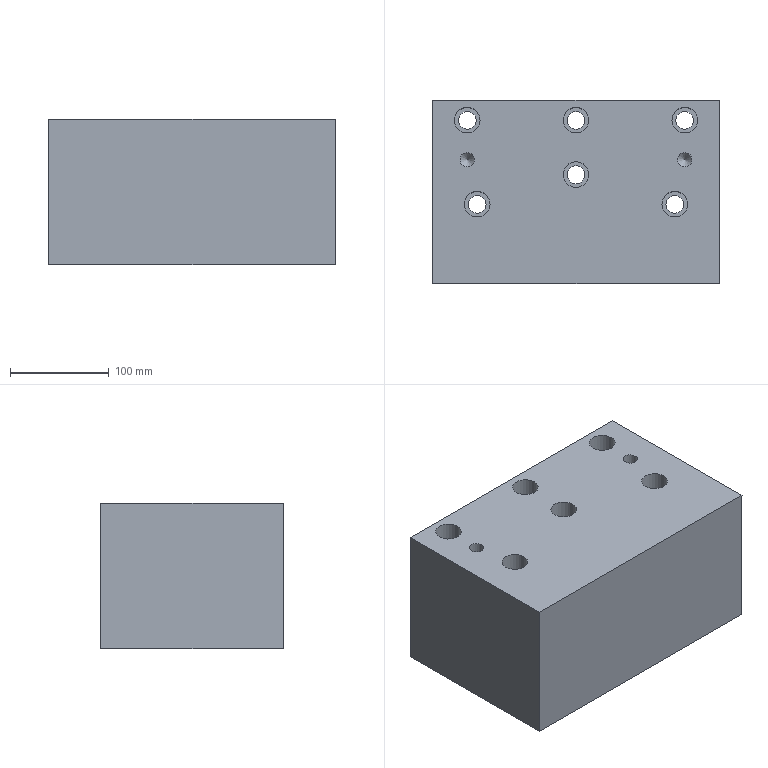Part | STEP file | lll_id2190_x_t | 1 solid | 32 faces | box 290 x 185 x 147.5 mm | volume 7467987 mm3 | cylinder 16 | plane 12 | cone 4 | commonest cylinder face diameters 18.009 x6 26.008 x6 14.506 x4
STEP:
#1=CARTESIAN_POINT('',(1973.431,-495.,262.5));
#2=VERTEX_POINT('',#1);
#3=CARTESIAN_POINT('',(1982.435,-495.,262.5));
#4=DIRECTION('',(0.,0.,-1.));
#5=DIRECTION('',(-1.,0.,0.));
#6=AXIS2_PLACEMENT_3D('',#3,#4,#5);
#7=CIRCLE('',#6,9.005);
#8=EDGE_CURVE('',#2,#2,#7,.T.);
#9=ORIENTED_EDGE('',*,*,#8,.T.);
#10=EDGE_LOOP('',(#9));
#11=FACE_BOUND('',#10,.T.);
#12=CARTESIAN_POINT('',(1995.439,-495.,262.5));
#13=VERTEX_POINT('',#12);
#14=CARTESIAN_POINT('',(1982.435,-495.,262.5));
#15=DIRECTION('',(0.,0.,-1.));
#16=DIRECTION('',(1.,0.,0.));
#17=AXIS2_PLACEMENT_3D('',#14,#15,#16);
#18=CIRCLE('',#17,13.004);
#19=EDGE_CURVE('',#13,#13,#18,.T.);
#20=ORIENTED_EDGE('',*,*,#19,.F.);
#21=EDGE_LOOP('',(#20));
#22=FACE_BOUND('',#21,.T.);
#23=CARTESIAN_POINT('',(1982.435,-495.,262.5));
#24=DIRECTION('',(0.,0.,-1.));
#25=DIRECTION('',(-1.,0.,0.));
#26=AXIS2_PLACEMENT_3D('',#23,#24,#25);
#27=PLANE('',#26);
#28=ADVANCED_FACE('',(#11,#22),#27,.F.);
#29=CARTESIAN_POINT('',(1983.431,-580.,262.5));
#30=VERTEX_POINT('',#29);
#31=CARTESIAN_POINT('',(1992.435,-580.,262.5));
#32=DIRECTION('',(0.,0.,-1.));
#33=DIRECTION('',(-1.,0.,0.));
#34=AXIS2_PLACEMENT_3D('',#31,#32,#33);
#35=CIRCLE('',#34,9.005);
#36=EDGE_CURVE('',#30,#30,#35,.T.);
#37=ORIENTED_EDGE('',*,*,#36,.T.);
#38=EDGE_LOOP('',(#37));
#39=FACE_BOUND('',#38,.T.);
#40=CARTESIAN_POINT('',(2005.439,-580.,262.5));
#41=VERTEX_POINT('',#40);
#42=CARTESIAN_POINT('',(1992.435,-580.,262.5));
#43=DIRECTION('',(0.,0.,-1.));
#44=DIRECTION('',(1.,0.,0.));
#45=AXIS2_PLACEMENT_3D('',#42,#43,#44);
#46=CIRCLE('',#45,13.004);
#47=EDGE_CURVE('',#41,#41,#46,.T.);
#48=ORIENTED_EDGE('',*,*,#47,.F.);
#49=EDGE_LOOP('',(#48));
#50=FACE_BOUND('',#49,.T.);
#51=CARTESIAN_POINT('',(1992.435,-580.,262.5));
#52=DIRECTION('',(0.,0.,-1.));
#53=DIRECTION('',(-1.,0.,0.));
#54=AXIS2_PLACEMENT_3D('',#51,#52,#53);
#55=PLANE('',#54);
#56=ADVANCED_FACE('',(#39,#50),#55,.F.);
#57=CARTESIAN_POINT('',(1982.435,-535.,279.494));
#58=VERTEX_POINT('',#57);
#59=VERTEX_LOOP('',#58);
#60=FACE_BOUND('',#59,.T.);
#61=CARTESIAN_POINT('',(1989.688,-535.,286.747));
#62=VERTEX_POINT('',#61);
#63=CARTESIAN_POINT('',(1982.435,-535.,286.747));
#64=DIRECTION('',(0.,0.,-1.));
#65=DIRECTION('',(1.,0.,0.));
#66=AXIS2_PLACEMENT_3D('',#63,#64,#65);
#67=CIRCLE('',#66,7.253);
#68=EDGE_CURVE('',#62,#62,#67,.T.);
#69=ORIENTED_EDGE('',*,*,#68,.F.);
#70=EDGE_LOOP('',(#69));
#71=FACE_BOUND('',#70,.T.);
#72=CARTESIAN_POINT('',(1982.435,-535.,286.747));
#73=DIRECTION('',(0.,0.,1.));
#74=DIRECTION('',(-1.,0.,0.));
#75=AXIS2_PLACEMENT_3D('',#72,#73,#74);
#76=CONICAL_SURFACE('',#75,7.253,45.);
#77=ADVANCED_FACE('',(#60,#71),#76,.F.);
#78=CARTESIAN_POINT('',(2202.435,-535.,279.494));
#79=VERTEX_POINT('',#78);
#80=VERTEX_LOOP('',#79);
#81=FACE_BOUND('',#80,.T.);
#82=CARTESIAN_POINT('',(2195.182,-535.,286.747));
#83=VERTEX_POINT('',#82);
#84=CARTESIAN_POINT('',(2202.435,-535.,286.747));
#85=DIRECTION('',(0.,0.,-1.));
#86=DIRECTION('',(-1.,0.,0.));
#87=AXIS2_PLACEMENT_3D('',#84,#85,#86);
#88=CIRCLE('',#87,7.253);
#89=EDGE_CURVE('',#83,#83,#88,.T.);
#90=ORIENTED_EDGE('',*,*,#89,.F.);
#91=EDGE_LOOP('',(#90));
#92=FACE_BOUND('',#91,.T.);
#93=CARTESIAN_POINT('',(2202.435,-535.,286.747));
#94=DIRECTION('',(0.,0.,1.));
#95=DIRECTION('',(1.,0.,0.));
#96=AXIS2_PLACEMENT_3D('',#93,#94,#95);
#97=CONICAL_SURFACE('',#96,7.253,45.);
#98=ADVANCED_FACE('',(#81,#92),#97,.F.);
#99=CARTESIAN_POINT('',(2211.44,-495.,262.5));
#100=VERTEX_POINT('',#99);
#101=CARTESIAN_POINT('',(2202.435,-495.,262.5));
#102=DIRECTION('',(0.,0.,-1.));
#103=DIRECTION('',(1.,0.,0.));
#104=AXIS2_PLACEMENT_3D('',#101,#102,#103);
#105=CIRCLE('',#104,9.005);
#106=EDGE_CURVE('',#100,#100,#105,.T.);
#107=ORIENTED_EDGE('',*,*,#106,.T.);
#108=EDGE_LOOP('',(#107));
#109=FACE_BOUND('',#108,.T.);
#110=CARTESIAN_POINT('',(2189.431,-495.,262.5));
#111=VERTEX_POINT('',#110);
#112=CARTESIAN_POINT('',(2202.435,-495.,262.5));
#113=DIRECTION('',(0.,0.,-1.));
#114=DIRECTION('',(-1.,0.,0.));
#115=AXIS2_PLACEMENT_3D('',#112,#113,#114);
#116=CIRCLE('',#115,13.004);
#117=EDGE_CURVE('',#111,#111,#116,.T.);
#118=ORIENTED_EDGE('',*,*,#117,.F.);
#119=EDGE_LOOP('',(#118));
#120=FACE_BOUND('',#119,.T.);
#121=CARTESIAN_POINT('',(2202.435,-495.,262.5));
#122=DIRECTION('',(0.,0.,-1.));
#123=DIRECTION('',(1.,0.,0.));
#124=AXIS2_PLACEMENT_3D('',#121,#122,#123);
#125=PLANE('',#124);
#126=ADVANCED_FACE('',(#109,#120),#125,.F.);
#127=CARTESIAN_POINT('',(2201.44,-580.,262.5));
#128=VERTEX_POINT('',#127);
#129=CARTESIAN_POINT('',(2192.435,-580.,262.5));
#130=DIRECTION('',(0.,0.,-1.));
#131=DIRECTION('',(1.,0.,0.));
#132=AXIS2_PLACEMENT_3D('',#129,#130,#131);
#133=CIRCLE('',#132,9.005);
#134=EDGE_CURVE('',#128,#128,#133,.T.);
#135=ORIENTED_EDGE('',*,*,#134,.T.);
#136=EDGE_LOOP('',(#135));
#137=FACE_BOUND('',#136,.T.);
#138=CARTESIAN_POINT('',(2179.431,-580.,262.5));
#139=VERTEX_POINT('',#138);
#140=CARTESIAN_POINT('',(2192.435,-580.,262.5));
#141=DIRECTION('',(0.,0.,-1.));
#142=DIRECTION('',(-1.,0.,0.));
#143=AXIS2_PLACEMENT_3D('',#140,#141,#142);
#144=CIRCLE('',#143,13.004);
#145=EDGE_CURVE('',#139,#139,#144,.T.);
#146=ORIENTED_EDGE('',*,*,#145,.F.);
#147=EDGE_LOOP('',(#146));
#148=FACE_BOUND('',#147,.T.);
#149=CARTESIAN_POINT('',(2192.435,-580.,262.5));
#150=DIRECTION('',(0.,0.,-1.));
#151=DIRECTION('',(1.,0.,0.));
#152=AXIS2_PLACEMENT_3D('',#149,#150,#151);
#153=PLANE('',#152);
#154=ADVANCED_FACE('',(#137,#148),#153,.F.);
#155=ORIENTED_EDGE('',*,*,#19,.T.);
#156=EDGE_LOOP('',(#155));
#157=FACE_BOUND('',#156,.T.);
#158=CARTESIAN_POINT('',(1969.431,-495.,370.));
#159=VERTEX_POINT('',#158);
#160=CARTESIAN_POINT('',(1982.435,-495.,370.));
#161=DIRECTION('',(0.,0.,-1.));
#162=DIRECTION('',(-1.,0.,0.));
#163=AXIS2_PLACEMENT_3D('',#160,#161,#162);
#164=CIRCLE('',#163,13.004);
#165=EDGE_CURVE('',#159,#159,#164,.T.);
#166=ORIENTED_EDGE('',*,*,#165,.F.);
#167=EDGE_LOOP('',(#166));
#168=FACE_BOUND('',#167,.T.);
#169=CARTESIAN_POINT('',(1982.435,-495.,322.5));
#170=DIRECTION('',(0.,0.,-1.));
#171=DIRECTION('',(1.,0.,0.));
#172=AXIS2_PLACEMENT_3D('',#169,#170,#171);
#173=CYLINDRICAL_SURFACE('',#172,13.004);
#174=ADVANCED_FACE('',(#157,#168),#173,.F.);
#175=CARTESIAN_POINT('',(2237.435,-475.,222.5));
#176=VERTEX_POINT('',#175);
#177=CARTESIAN_POINT('',(2237.435,-475.,370.));
#178=VERTEX_POINT('',#177);
#179=CARTESIAN_POINT('',(2237.435,-475.,76.5));
#180=DIRECTION('',(0.,0.,1.));
#181=VECTOR('',#180,1.);
#182=LINE('',#179,#181);
#183=EDGE_CURVE('',#176,#178,#182,.T.);
#184=ORIENTED_EDGE('',*,*,#183,.T.);
#185=CARTESIAN_POINT('',(2237.435,-660.,370.));
#186=VERTEX_POINT('',#185);
#187=CARTESIAN_POINT('',(2237.435,-631.,370.));
#188=DIRECTION('',(0.,-1.,0.));
#189=VECTOR('',#188,1.);
#190=LINE('',#187,#189);
#191=EDGE_CURVE('',#178,#186,#190,.T.);
#192=ORIENTED_EDGE('',*,*,#191,.T.);
#193=CARTESIAN_POINT('',(2237.435,-660.,222.5));
#194=VERTEX_POINT('',#193);
#195=CARTESIAN_POINT('',(2237.435,-660.,76.5));
#196=DIRECTION('',(0.,-0.000000092,1.));
#197=VECTOR('',#196,1.);
#198=LINE('',#195,#197);
#199=EDGE_CURVE('',#194,#186,#198,.T.);
#200=ORIENTED_EDGE('',*,*,#199,.F.);
#201=CARTESIAN_POINT('',(2237.435,-631.,222.5));
#202=DIRECTION('',(0.,-1.,0.));
#203=VECTOR('',#202,1.);
#204=LINE('',#201,#203);
#205=EDGE_CURVE('',#176,#194,#204,.T.);
#206=ORIENTED_EDGE('',*,*,#205,.F.);
#207=EDGE_LOOP('',(#184,#192,#200,#206));
#208=FACE_OUTER_BOUND('',#207,.T.);
#209=CARTESIAN_POINT('',(2237.435,-631.,76.5));
#210=DIRECTION('',(-1.,0.,0.));
#211=DIRECTION('',(0.,-0.000000092,1.));
#212=AXIS2_PLACEMENT_3D('',#209,#210,#211);
#213=PLANE('',#212);
#214=ADVANCED_FACE('',(#208),#213,.F.);
#215=CARTESIAN_POINT('',(1947.435,-475.,222.5));
#216=VERTEX_POINT('',#215);
#217=CARTESIAN_POINT('',(1947.435,-475.,370.));
#218=VERTEX_POINT('',#217);
#219=CARTESIAN_POINT('',(1947.435,-475.,157.5));
#220=DIRECTION('',(0.,0.,1.));
#221=VECTOR('',#220,1.);
#222=LINE('',#219,#221);
#223=EDGE_CURVE('',#216,#218,#222,.T.);
#224=ORIENTED_EDGE('',*,*,#223,.T.);
#225=CARTESIAN_POINT('',(2092.435,-475.,370.));
#226=DIRECTION('',(-1.,0.,0.));
#227=VECTOR('',#226,1.);
#228=LINE('',#225,#227);
#229=EDGE_CURVE('',#178,#218,#228,.T.);
#230=ORIENTED_EDGE('',*,*,#229,.F.);
#231=ORIENTED_EDGE('',*,*,#183,.F.);
#232=CARTESIAN_POINT('',(2092.435,-475.,222.5));
#233=DIRECTION('',(-1.,0.,0.));
#234=VECTOR('',#233,1.);
#235=LINE('',#232,#234);
#236=EDGE_CURVE('',#176,#216,#235,.T.);
#237=ORIENTED_EDGE('',*,*,#236,.T.);
#238=EDGE_LOOP('',(#224,#230,#231,#237));
#239=FACE_OUTER_BOUND('',#238,.T.);
#240=CARTESIAN_POINT('',(2092.435,-475.,157.5));
#241=DIRECTION('',(0.,1.,0.));
#242=DIRECTION('',(0.,0.,1.));
#243=AXIS2_PLACEMENT_3D('',#240,#241,#242);
#244=PLANE('',#243);
#245=ADVANCED_FACE('',(#239),#244,.T.);
#246=CARTESIAN_POINT('',(1947.435,-660.,222.5));
#247=VERTEX_POINT('',#246);
#248=CARTESIAN_POINT('',(1947.435,-660.,370.));
#249=VERTEX_POINT('',#248);
#250=CARTESIAN_POINT('',(1947.435,-660.,76.5));
#251=DIRECTION('',(0.,-0.000000092,1.));
#252=VECTOR('',#251,1.);
#253=LINE('',#250,#252);
#254=EDGE_CURVE('',#247,#249,#253,.T.);
#255=ORIENTED_EDGE('',*,*,#254,.T.);
#256=CARTESIAN_POINT('',(1947.435,-551.,370.));
#257=DIRECTION('',(0.,1.,0.));
#258=VECTOR('',#257,1.);
#259=LINE('',#256,#258);
#260=EDGE_CURVE('',#249,#218,#259,.T.);
#261=ORIENTED_EDGE('',*,*,#260,.T.);
#262=ORIENTED_EDGE('',*,*,#223,.F.);
#263=CARTESIAN_POINT('',(1947.435,-551.,222.5));
#264=DIRECTION('',(0.,1.,0.));
#265=VECTOR('',#264,1.);
#266=LINE('',#263,#265);
#267=EDGE_CURVE('',#247,#216,#266,.T.);
#268=ORIENTED_EDGE('',*,*,#267,.F.);
#269=EDGE_LOOP('',(#255,#261,#262,#268));
#270=FACE_OUTER_BOUND('',#269,.T.);
#271=CARTESIAN_POINT('',(1947.435,-551.,76.5));
#272=DIRECTION('',(1.,0.,0.));
#273=DIRECTION('',(0.,0.000000092,-1.));
#274=AXIS2_PLACEMENT_3D('',#271,#272,#273);
#275=PLANE('',#274);
#276=ADVANCED_FACE('',(#270),#275,.F.);
#277=ORIENTED_EDGE('',*,*,#199,.T.);
#278=CARTESIAN_POINT('',(-319.315,-660.,370.));
#279=DIRECTION('',(-1.,0.,0.));
#280=VECTOR('',#279,1.);
#281=LINE('',#278,#280);
#282=EDGE_CURVE('',#186,#249,#281,.T.);
#283=ORIENTED_EDGE('',*,*,#282,.T.);
#284=ORIENTED_EDGE('',*,*,#254,.F.);
#285=CARTESIAN_POINT('',(2067.435,-660.,222.5));
#286=DIRECTION('',(-1.,0.,0.));
#287=VECTOR('',#286,1.);
#288=LINE('',#285,#287);
#289=EDGE_CURVE('',#194,#247,#288,.T.);
#290=ORIENTED_EDGE('',*,*,#289,.F.);
#291=EDGE_LOOP('',(#277,#283,#284,#290));
#292=FACE_OUTER_BOUND('',#291,.T.);
#293=CARTESIAN_POINT('',(1972.935,-660.,76.5));
#294=DIRECTION('',(0.,1.,0.000000092));
#295=DIRECTION('',(-1.,0.,0.));
#296=AXIS2_PLACEMENT_3D('',#293,#294,#295);
#297=PLANE('',#296);
#298=ADVANCED_FACE('',(#292),#297,.F.);
#299=ORIENTED_EDGE('',*,*,#47,.T.);
#300=EDGE_LOOP('',(#299));
#301=FACE_BOUND('',#300,.T.);
#302=CARTESIAN_POINT('',(1979.431,-580.,370.));
#303=VERTEX_POINT('',#302);
#304=CARTESIAN_POINT('',(1992.435,-580.,370.));
#305=DIRECTION('',(0.,0.,-1.));
#306=DIRECTION('',(-1.,0.,0.));
#307=AXIS2_PLACEMENT_3D('',#304,#305,#306);
#308=CIRCLE('',#307,13.004);
#309=EDGE_CURVE('',#303,#303,#308,.T.);
#310=ORIENTED_EDGE('',*,*,#309,.F.);
#311=EDGE_LOOP('',(#310));
#312=FACE_BOUND('',#311,.T.);
#313=CARTESIAN_POINT('',(1992.435,-580.,322.5));
#314=DIRECTION('',(0.,0.,-1.));
#315=DIRECTION('',(1.,0.,0.));
#316=AXIS2_PLACEMENT_3D('',#313,#314,#315);
#317=CYLINDRICAL_SURFACE('',#316,13.004);
#318=ADVANCED_FACE('',(#301,#312),#317,.F.);
#319=CARTESIAN_POINT('',(1975.182,-535.,370.));
#320=VERTEX_POINT('',#319);
#321=CARTESIAN_POINT('',(1982.435,-535.,370.));
#322=DIRECTION('',(0.,0.,1.));
#323=DIRECTION('',(-1.,0.,0.));
#324=AXIS2_PLACEMENT_3D('',#321,#322,#323);
#325=CIRCLE('',#324,7.253);
#326=EDGE_CURVE('',#320,#320,#325,.T.);
#327=ORIENTED_EDGE('',*,*,#326,.T.);
#328=EDGE_LOOP('',(#327));
#329=FACE_BOUND('',#328,.T.);
#330=ORIENTED_EDGE('',*,*,#68,.T.);
#331=EDGE_LOOP('',(#330));
#332=FACE_BOUND('',#331,.T.);
#333=CARTESIAN_POINT('',(1982.435,-535.,324.5));
#334=DIRECTION('',(0.,0.,-1.));
#335=DIRECTION('',(-1.,0.,0.));
#336=AXIS2_PLACEMENT_3D('',#333,#334,#335);
#337=CYLINDRICAL_SURFACE('',#336,7.253);
#338=ADVANCED_FACE('',(#329,#332),#337,.F.);
#339=CARTESIAN_POINT('',(2195.182,-535.,370.));
#340=VERTEX_POINT('',#339);
#341=CARTESIAN_POINT('',(2202.435,-535.,370.));
#342=DIRECTION('',(0.,0.,-1.));
#343=DIRECTION('',(-1.,0.,0.));
#344=AXIS2_PLACEMENT_3D('',#341,#342,#343);
#345=CIRCLE('',#344,7.253);
#346=EDGE_CURVE('',#340,#340,#345,.T.);
#347=ORIENTED_EDGE('',*,*,#346,.F.);
#348=EDGE_LOOP('',(#347));
#349=FACE_BOUND('',#348,.T.);
#350=ORIENTED_EDGE('',*,*,#89,.T.);
#351=EDGE_LOOP('',(#350));
#352=FACE_BOUND('',#351,.T.);
#353=CARTESIAN_POINT('',(2202.435,-535.,324.5));
#354=DIRECTION('',(0.,0.,-1.));
#355=DIRECTION('',(1.,0.,0.));
#356=AXIS2_PLACEMENT_3D('',#353,#354,#355);
#357=CYLINDRICAL_SURFACE('',#356,7.253);
#358=ADVANCED_FACE('',(#349,#352),#357,.F.);
#359=ORIENTED_EDGE('',*,*,#117,.T.);
#360=EDGE_LOOP('',(#359));
#361=FACE_BOUND('',#360,.T.);
#362=CARTESIAN_POINT('',(2189.431,-495.,370.));
#363=VERTEX_POINT('',#362);
#364=CARTESIAN_POINT('',(2202.435,-495.,370.));
#365=DIRECTION('',(0.,0.,-1.));
#366=DIRECTION('',(-1.,0.,0.));
#367=AXIS2_PLACEMENT_3D('',#364,#365,#366);
#368=CIRCLE('',#367,13.004);
#369=EDGE_CURVE('',#363,#363,#368,.T.);
#370=ORIENTED_EDGE('',*,*,#369,.F.);
#371=EDGE_LOOP('',(#370));
#372=FACE_BOUND('',#371,.T.);
#373=CARTESIAN_POINT('',(2202.435,-495.,322.5));
#374=DIRECTION('',(0.,0.,-1.));
#375=DIRECTION('',(-1.,0.,0.));
#376=AXIS2_PLACEMENT_3D('',#373,#374,#375);
#377=CYLINDRICAL_SURFACE('',#376,13.004);
#378=ADVANCED_FACE('',(#361,#372),#377,.F.);
#379=ORIENTED_EDGE('',*,*,#145,.T.);
#380=EDGE_LOOP('',(#379));
#381=FACE_BOUND('',#380,.T.);
#382=CARTESIAN_POINT('',(2179.431,-580.,370.));
#383=VERTEX_POINT('',#382);
#384=CARTESIAN_POINT('',(2192.435,-580.,370.));
#385=DIRECTION('',(0.,0.,-1.));
#386=DIRECTION('',(-1.,0.,0.));
#387=AXIS2_PLACEMENT_3D('',#384,#385,#386);
#388=CIRCLE('',#387,13.004);
#389=EDGE_CURVE('',#383,#383,#388,.T.);
#390=ORIENTED_EDGE('',*,*,#389,.F.);
#391=EDGE_LOOP('',(#390));
#392=FACE_BOUND('',#391,.T.);
#393=CARTESIAN_POINT('',(2192.435,-580.,322.5));
#394=DIRECTION('',(0.,0.,-1.));
#395=DIRECTION('',(-1.,0.,0.));
#396=AXIS2_PLACEMENT_3D('',#393,#394,#395);
#397=CYLINDRICAL_SURFACE('',#396,13.004);
#398=ADVANCED_FACE('',(#381,#392),#397,.F.);
#399=CARTESIAN_POINT('',(2079.431,-495.,370.));
#400=VERTEX_POINT('',#399);
#401=CARTESIAN_POINT('',(2092.435,-495.,370.));
#402=DIRECTION('',(0.,0.,-1.));
#403=DIRECTION('',(-1.,0.,0.));
#404=AXIS2_PLACEMENT_3D('',#401,#402,#403);
#405=CIRCLE('',#404,13.004);
#406=EDGE_CURVE('',#400,#400,#405,.T.);
#407=ORIENTED_EDGE('',*,*,#406,.T.);
#408=EDGE_LOOP('',(#407));
#409=FACE_BOUND('',#408,.T.);
#410=CARTESIAN_POINT('',(2079.431,-550.,370.));
#411=VERTEX_POINT('',#410);
#412=CARTESIAN_POINT('',(2092.435,-550.,370.));
#413=DIRECTION('',(0.,0.,-1.));
#414=DIRECTION('',(-1.,0.,0.));
#415=AXIS2_PLACEMENT_3D('',#412,#413,#414);
#416=CIRCLE('',#415,13.004);
#417=EDGE_CURVE('',#411,#411,#416,.T.);
#418=ORIENTED_EDGE('',*,*,#417,.T.);
#419=EDGE_LOOP('',(#418));
#420=FACE_BOUND('',#419,.T.);
#421=ORIENTED_EDGE('',*,*,#389,.T.);
#422=EDGE_LOOP('',(#421));
#423=FACE_BOUND('',#422,.T.);
#424=ORIENTED_EDGE('',*,*,#369,.T.);
#425=EDGE_LOOP('',(#424));
#426=FACE_BOUND('',#425,.T.);
#427=ORIENTED_EDGE('',*,*,#346,.T.);
#428=EDGE_LOOP('',(#427));
#429=FACE_BOUND('',#428,.T.);
#430=ORIENTED_EDGE('',*,*,#326,.F.);
#431=EDGE_LOOP('',(#430));
#432=FACE_BOUND('',#431,.T.);
#433=ORIENTED_EDGE('',*,*,#309,.T.);
#434=EDGE_LOOP('',(#433));
#435=FACE_BOUND('',#434,.T.);
#436=ORIENTED_EDGE('',*,*,#282,.F.);
#437=ORIENTED_EDGE('',*,*,#191,.F.);
#438=ORIENTED_EDGE('',*,*,#229,.T.);
#439=ORIENTED_EDGE('',*,*,#260,.F.);
#440=EDGE_LOOP('',(#436,#437,#438,#439));
#441=FACE_BOUND('',#440,.T.);
#442=ORIENTED_EDGE('',*,*,#165,.T.);
#443=EDGE_LOOP('',(#442));
#444=FACE_BOUND('',#443,.T.);
#445=CARTESIAN_POINT('',(-319.315,-1.,370.));
#446=DIRECTION('',(0.,0.,-1.));
#447=DIRECTION('',(1.,0.,0.));
#448=AXIS2_PLACEMENT_3D('',#445,#446,#447);
#449=PLANE('',#448);
#450=ADVANCED_FACE('',(#409,#420,#423,#426,#429,#432,#435,#441,#444),#449,.F.);
#451=ORIENTED_EDGE('',*,*,#36,.F.);
#452=EDGE_LOOP('',(#451));
#453=FACE_BOUND('',#452,.T.);
#454=CARTESIAN_POINT('',(2001.44,-580.,222.5));
#455=VERTEX_POINT('',#454);
#456=CARTESIAN_POINT('',(1992.435,-580.,222.5));
#457=DIRECTION('',(0.,0.,1.));
#458=DIRECTION('',(1.,0.,0.));
#459=AXIS2_PLACEMENT_3D('',#456,#457,#458);
#460=CIRCLE('',#459,9.005);
#461=EDGE_CURVE('',#455,#455,#460,.T.);
#462=ORIENTED_EDGE('',*,*,#461,.F.);
#463=EDGE_LOOP('',(#462));
#464=FACE_BOUND('',#463,.T.);
#465=CARTESIAN_POINT('',(1992.435,-580.,324.5));
#466=DIRECTION('',(0.,0.,-1.));
#467=DIRECTION('',(1.,0.,0.));
#468=AXIS2_PLACEMENT_3D('',#465,#466,#467);
#469=CYLINDRICAL_SURFACE('',#468,9.005);
#470=ADVANCED_FACE('',(#453,#464),#469,.F.);
#471=ORIENTED_EDGE('',*,*,#8,.F.);
#472=EDGE_LOOP('',(#471));
#473=FACE_BOUND('',#472,.T.);
#474=CARTESIAN_POINT('',(1991.44,-495.,222.5));
#475=VERTEX_POINT('',#474);
#476=CARTESIAN_POINT('',(1982.435,-495.,222.5));
#477=DIRECTION('',(0.,0.,1.));
#478=DIRECTION('',(1.,0.,0.));
#479=AXIS2_PLACEMENT_3D('',#476,#477,#478);
#480=CIRCLE('',#479,9.005);
#481=EDGE_CURVE('',#475,#475,#480,.T.);
#482=ORIENTED_EDGE('',*,*,#481,.F.);
#483=EDGE_LOOP('',(#482));
#484=FACE_BOUND('',#483,.T.);
#485=CARTESIAN_POINT('',(1982.435,-495.,324.5));
#486=DIRECTION('',(0.,0.,-1.));
#487=DIRECTION('',(1.,0.,0.));
#488=AXIS2_PLACEMENT_3D('',#485,#486,#487);
#489=CYLINDRICAL_SURFACE('',#488,9.005);
#490=ADVANCED_FACE('',(#473,#484),#489,.F.);
#491=ORIENTED_EDGE('',*,*,#106,.F.);
#492=EDGE_LOOP('',(#491));
#493=FACE_BOUND('',#492,.T.);
#494=CARTESIAN_POINT('',(2211.44,-495.,222.5));
#495=VERTEX_POINT('',#494);
#496=CARTESIAN_POINT('',(2202.435,-495.,222.5));
#497=DIRECTION('',(0.,0.,-1.));
#498=DIRECTION('',(1.,0.,0.));
#499=AXIS2_PLACEMENT_3D('',#496,#497,#498);
#500=CIRCLE('',#499,9.005);
#501=EDGE_CURVE('',#495,#495,#500,.T.);
#502=ORIENTED_EDGE('',*,*,#501,.T.);
#503=EDGE_LOOP('',(#502));
#504=FACE_BOUND('',#503,.T.);
#505=CARTESIAN_POINT('',(2202.435,-495.,324.5));
#506=DIRECTION('',(0.,0.,-1.));
#507=DIRECTION('',(-1.,0.,0.));
#508=AXIS2_PLACEMENT_3D('',#505,#506,#507);
#509=CYLINDRICAL_SURFACE('',#508,9.005);
#510=ADVANCED_FACE('',(#493,#504),#509,.F.);
#511=ORIENTED_EDGE('',*,*,#134,.F.);
#512=EDGE_LOOP('',(#511));
#513=FACE_BOUND('',#512,.T.);
#514=CARTESIAN_POINT('',(2201.44,-580.,222.5));
#515=VERTEX_POINT('',#514);
#516=CARTESIAN_POINT('',(2192.435,-580.,222.5));
#517=DIRECTION('',(0.,0.,-1.));
#518=DIRECTION('',(1.,0.,0.));
#519=AXIS2_PLACEMENT_3D('',#516,#517,#518);
#520=CIRCLE('',#519,9.005);
#521=EDGE_CURVE('',#515,#515,#520,.T.);
#522=ORIENTED_EDGE('',*,*,#521,.T.);
#523=EDGE_LOOP('',(#522));
#524=FACE_BOUND('',#523,.T.);
#525=CARTESIAN_POINT('',(2192.435,-580.,324.5));
#526=DIRECTION('',(0.,0.,-1.));
#527=DIRECTION('',(-1.,0.,0.));
#528=AXIS2_PLACEMENT_3D('',#525,#526,#527);
#529=CYLINDRICAL_SURFACE('',#528,9.005);
#530=ADVANCED_FACE('',(#513,#524),#529,.F.);
#531=CARTESIAN_POINT('',(2190.688,-620.,222.5));
#532=VERTEX_POINT('',#531);
#533=CARTESIAN_POINT('',(2183.435,-620.,222.5));
#534=DIRECTION('',(0.,0.,1.));
#535=DIRECTION('',(1.,0.,0.));
#536=AXIS2_PLACEMENT_3D('',#533,#534,#535);
#537=CIRCLE('',#536,7.253);
#538=EDGE_CURVE('',#532,#532,#537,.T.);
#539=ORIENTED_EDGE('',*,*,#538,.T.);
#540=EDGE_LOOP('',(#539));
#541=FACE_BOUND('',#540,.T.);
#542=CARTESIAN_POINT('',(2008.688,-630.,222.5));
#543=VERTEX_POINT('',#542);
#544=CARTESIAN_POINT('',(2001.435,-630.,222.5));
#545=DIRECTION('',(0.,0.,1.));
#546=DIRECTION('',(1.,0.,0.));
#547=AXIS2_PLACEMENT_3D('',#544,#545,#546);
#548=CIRCLE('',#547,7.253);
#549=EDGE_CURVE('',#543,#543,#548,.T.);
#550=ORIENTED_EDGE('',*,*,#549,.T.);
#551=EDGE_LOOP('',(#550));
#552=FACE_BOUND('',#551,.T.);
#553=CARTESIAN_POINT('',(2101.44,-495.,222.5));
#554=VERTEX_POINT('',#553);
#555=CARTESIAN_POINT('',(2092.435,-495.,222.5));
#556=DIRECTION('',(0.,0.,-1.));
#557=DIRECTION('',(1.,0.,0.));
#558=AXIS2_PLACEMENT_3D('',#555,#556,#557);
#559=CIRCLE('',#558,9.005);
#560=EDGE_CURVE('',#554,#554,#559,.T.);
#561=ORIENTED_EDGE('',*,*,#560,.F.);
#562=EDGE_LOOP('',(#561));
#563=FACE_BOUND('',#562,.T.);
#564=CARTESIAN_POINT('',(2101.44,-550.,222.5));
#565=VERTEX_POINT('',#564);
#566=CARTESIAN_POINT('',(2092.435,-550.,222.5));
#567=DIRECTION('',(0.,0.,-1.));
#568=DIRECTION('',(1.,0.,0.));
#569=AXIS2_PLACEMENT_3D('',#566,#567,#568);
#570=CIRCLE('',#569,9.005);
#571=EDGE_CURVE('',#565,#565,#570,.T.);
#572=ORIENTED_EDGE('',*,*,#571,.F.);
#573=EDGE_LOOP('',(#572));
#574=FACE_BOUND('',#573,.T.);
#575=ORIENTED_EDGE('',*,*,#521,.F.);
#576=EDGE_LOOP('',(#575));
#577=FACE_BOUND('',#576,.T.);
#578=ORIENTED_EDGE('',*,*,#501,.F.);
#579=EDGE_LOOP('',(#578));
#580=FACE_BOUND('',#579,.T.);
#581=ORIENTED_EDGE('',*,*,#481,.T.);
#582=EDGE_LOOP('',(#581));
#583=FACE_BOUND('',#582,.T.);
#584=ORIENTED_EDGE('',*,*,#461,.T.);
#585=EDGE_LOOP('',(#584));
#586=FACE_BOUND('',#585,.T.);
#587=ORIENTED_EDGE('',*,*,#289,.T.);
#588=ORIENTED_EDGE('',*,*,#267,.T.);
#589=ORIENTED_EDGE('',*,*,#236,.F.);
#590=ORIENTED_EDGE('',*,*,#205,.T.);
#591=EDGE_LOOP('',(#587,#588,#589,#590));
#592=FACE_BOUND('',#591,.T.);
#593=CARTESIAN_POINT('',(2067.435,-0.000025,222.5));
#594=DIRECTION('',(0.,0.,1.));
#595=DIRECTION('',(1.,0.,0.));
#596=AXIS2_PLACEMENT_3D('',#593,#594,#595);
#597=PLANE('',#596);
#598=ADVANCED_FACE('',(#541,#552,#563,#574,#577,#580,#583,#586,#592),#597,.F.);
#599=CARTESIAN_POINT('',(2083.431,-550.,262.5));
#600=VERTEX_POINT('',#599);
#601=CARTESIAN_POINT('',(2092.435,-550.,262.5));
#602=DIRECTION('',(0.,0.,-1.));
#603=DIRECTION('',(-1.,0.,0.));
#604=AXIS2_PLACEMENT_3D('',#601,#602,#603);
#605=CIRCLE('',#604,9.005);
#606=EDGE_CURVE('',#600,#600,#605,.T.);
#607=ORIENTED_EDGE('',*,*,#606,.T.);
#608=EDGE_LOOP('',(#607));
#609=FACE_BOUND('',#608,.T.);
#610=CARTESIAN_POINT('',(2105.439,-550.,262.5));
#611=VERTEX_POINT('',#610);
#612=CARTESIAN_POINT('',(2092.435,-550.,262.5));
#613=DIRECTION('',(0.,0.,-1.));
#614=DIRECTION('',(1.,0.,0.));
#615=AXIS2_PLACEMENT_3D('',#612,#613,#614);
#616=CIRCLE('',#615,13.004);
#617=EDGE_CURVE('',#611,#611,#616,.T.);
#618=ORIENTED_EDGE('',*,*,#617,.F.);
#619=EDGE_LOOP('',(#618));
#620=FACE_BOUND('',#619,.T.);
#621=CARTESIAN_POINT('',(2092.435,-580.,262.5));
#622=DIRECTION('',(0.,0.,-1.));
#623=DIRECTION('',(-1.,0.,0.));
#624=AXIS2_PLACEMENT_3D('',#621,#622,#623);
#625=PLANE('',#624);
#626=ADVANCED_FACE('',(#609,#620),#625,.F.);
#627=ORIENTED_EDGE('',*,*,#617,.T.);
#628=EDGE_LOOP('',(#627));
#629=FACE_BOUND('',#628,.T.);
#630=ORIENTED_EDGE('',*,*,#417,.F.);
#631=EDGE_LOOP('',(#630));
#632=FACE_BOUND('',#631,.T.);
#633=CARTESIAN_POINT('',(2092.435,-550.,322.5));
#634=DIRECTION('',(0.,0.,-1.));
#635=DIRECTION('',(1.,0.,0.));
#636=AXIS2_PLACEMENT_3D('',#633,#634,#635);
#637=CYLINDRICAL_SURFACE('',#636,13.004);
#638=ADVANCED_FACE('',(#629,#632),#637,.F.);
#639=ORIENTED_EDGE('',*,*,#606,.F.);
#640=EDGE_LOOP('',(#639));
#641=FACE_BOUND('',#640,.T.);
#642=ORIENTED_EDGE('',*,*,#571,.T.);
#643=EDGE_LOOP('',(#642));
#644=FACE_BOUND('',#643,.T.);
#645=CARTESIAN_POINT('',(2092.435,-550.,324.5));
#646=DIRECTION('',(0.,0.,-1.));
#647=DIRECTION('',(1.,0.,0.));
#648=AXIS2_PLACEMENT_3D('',#645,#646,#647);
#649=CYLINDRICAL_SURFACE('',#648,9.005);
#650=ADVANCED_FACE('',(#641,#644),#649,.F.);
#651=CARTESIAN_POINT('',(2083.431,-495.,262.5));
#652=VERTEX_POINT('',#651);
#653=CARTESIAN_POINT('',(2092.435,-495.,262.5));
#654=DIRECTION('',(0.,0.,-1.));
#655=DIRECTION('',(-1.,0.,0.));
#656=AXIS2_PLACEMENT_3D('',#653,#654,#655);
#657=CIRCLE('',#656,9.005);
#658=EDGE_CURVE('',#652,#652,#657,.T.);
#659=ORIENTED_EDGE('',*,*,#658,.T.);
#660=EDGE_LOOP('',(#659));
#661=FACE_BOUND('',#660,.T.);
#662=CARTESIAN_POINT('',(2105.439,-495.,262.5));
#663=VERTEX_POINT('',#662);
#664=CARTESIAN_POINT('',(2092.435,-495.,262.5));
#665=DIRECTION('',(0.,0.,-1.));
#666=DIRECTION('',(1.,0.,0.));
#667=AXIS2_PLACEMENT_3D('',#664,#665,#666);
#668=CIRCLE('',#667,13.004);
#669=EDGE_CURVE('',#663,#663,#668,.T.);
#670=ORIENTED_EDGE('',*,*,#669,.F.);
#671=EDGE_LOOP('',(#670));
#672=FACE_BOUND('',#671,.T.);
#673=CARTESIAN_POINT('',(2092.435,-495.,262.5));
#674=DIRECTION('',(0.,0.,-1.));
#675=DIRECTION('',(-1.,0.,0.));
#676=AXIS2_PLACEMENT_3D('',#673,#674,#675);
#677=PLANE('',#676);
#678=ADVANCED_FACE('',(#661,#672),#677,.F.);
#679=ORIENTED_EDGE('',*,*,#669,.T.);
#680=EDGE_LOOP('',(#679));
#681=FACE_BOUND('',#680,.T.);
#682=ORIENTED_EDGE('',*,*,#406,.F.);
#683=EDGE_LOOP('',(#682));
#684=FACE_BOUND('',#683,.T.);
#685=CARTESIAN_POINT('',(2092.435,-495.,322.5));
#686=DIRECTION('',(0.,0.,-1.));
#687=DIRECTION('',(1.,0.,0.));
#688=AXIS2_PLACEMENT_3D('',#685,#686,#687);
#689=CYLINDRICAL_SURFACE('',#688,13.004);
#690=ADVANCED_FACE('',(#681,#684),#689,.F.);
#691=ORIENTED_EDGE('',*,*,#658,.F.);
#692=EDGE_LOOP('',(#691));
#693=FACE_BOUND('',#692,.T.);
#694=ORIENTED_EDGE('',*,*,#560,.T.);
#695=EDGE_LOOP('',(#694));
#696=FACE_BOUND('',#695,.T.);
#697=CARTESIAN_POINT('',(2092.435,-495.,324.5));
#698=DIRECTION('',(0.,0.,-1.));
#699=DIRECTION('',(1.,0.,0.));
#700=AXIS2_PLACEMENT_3D('',#697,#698,#699);
#701=CYLINDRICAL_SURFACE('',#700,9.005);
#702=ADVANCED_FACE('',(#693,#696),#701,.F.);
#703=CARTESIAN_POINT('',(2008.688,-630.,260.253));
#704=VERTEX_POINT('',#703);
#705=CARTESIAN_POINT('',(2001.435,-630.,260.253));
#706=DIRECTION('',(0.,0.,1.));
#707=DIRECTION('',(1.,0.,0.));
#708=AXIS2_PLACEMENT_3D('',#705,#706,#707);
#709=CIRCLE('',#708,7.253);
#710=EDGE_CURVE('',#704,#704,#709,.T.);
#711=ORIENTED_EDGE('',*,*,#710,.T.);
#712=EDGE_LOOP('',(#711));
#713=FACE_BOUND('',#712,.T.);
#714=ORIENTED_EDGE('',*,*,#549,.F.);
#715=EDGE_LOOP('',(#714));
#716=FACE_BOUND('',#715,.T.);
#717=CARTESIAN_POINT('',(2001.435,-630.,222.5));
#718=DIRECTION('',(0.,0.,1.));
#719=DIRECTION('',(-1.,0.,0.));
#720=AXIS2_PLACEMENT_3D('',#717,#718,#719);
#721=CYLINDRICAL_SURFACE('',#720,7.253);
#722=ADVANCED_FACE('',(#713,#716),#721,.F.);
#723=CARTESIAN_POINT('',(2001.435,-630.,267.506));
#724=VERTEX_POINT('',#723);
#725=VERTEX_LOOP('',#724);
#726=FACE_BOUND('',#725,.T.);
#727=ORIENTED_EDGE('',*,*,#710,.F.);
#728=EDGE_LOOP('',(#727));
#729=FACE_BOUND('',#728,.T.);
#730=CARTESIAN_POINT('',(2001.435,-630.,260.253));
#731=DIRECTION('',(0.,0.,-1.));
#732=DIRECTION('',(1.,0.,0.));
#733=AXIS2_PLACEMENT_3D('',#730,#731,#732);
#734=CONICAL_SURFACE('',#733,7.253,45.);
#735=ADVANCED_FACE('',(#726,#729),#734,.F.);
#736=CARTESIAN_POINT('',(2190.688,-620.,260.253));
#737=VERTEX_POINT('',#736);
#738=CARTESIAN_POINT('',(2183.435,-620.,260.253));
#739=DIRECTION('',(0.,0.,1.));
#740=DIRECTION('',(1.,0.,0.));
#741=AXIS2_PLACEMENT_3D('',#738,#739,#740);
#742=CIRCLE('',#741,7.253);
#743=EDGE_CURVE('',#737,#737,#742,.T.);
#744=ORIENTED_EDGE('',*,*,#743,.T.);
#745=EDGE_LOOP('',(#744));
#746=FACE_BOUND('',#745,.T.);
#747=ORIENTED_EDGE('',*,*,#538,.F.);
#748=EDGE_LOOP('',(#747));
#749=FACE_BOUND('',#748,.T.);
#750=CARTESIAN_POINT('',(2183.435,-620.,222.5));
#751=DIRECTION('',(0.,0.,1.));
#752=DIRECTION('',(-1.,0.,0.));
#753=AXIS2_PLACEMENT_3D('',#750,#751,#752);
#754=CYLINDRICAL_SURFACE('',#753,7.253);
#755=ADVANCED_FACE('',(#746,#749),#754,.F.);
#756=CARTESIAN_POINT('',(2183.435,-620.,267.506));
#757=VERTEX_POINT('',#756);
#758=VERTEX_LOOP('',#757);
#759=FACE_BOUND('',#758,.T.);
#760=ORIENTED_EDGE('',*,*,#743,.F.);
#761=EDGE_LOOP('',(#760));
#762=FACE_BOUND('',#761,.T.);
#763=CARTESIAN_POINT('',(2183.435,-620.,260.253));
#764=DIRECTION('',(0.,0.,-1.));
#765=DIRECTION('',(1.,0.,0.));
#766=AXIS2_PLACEMENT_3D('',#763,#764,#765);
#767=CONICAL_SURFACE('',#766,7.253,45.);
#768=ADVANCED_FACE('',(#759,#762),#767,.F.);
#769=CLOSED_SHELL('',(#28,#56,#77,#98,#126,#154,#174,#214,#245,#276,#298,#318,#338,#358,#378,#398,#450,#470,#490,#510,#530,#598,#626,#638,#650,#678,#690,#702,#722,#735,#755,#768));
#770=MANIFOLD_SOLID_BREP('',#769);
#771=(LENGTH_UNIT()NAMED_UNIT(*)SI_UNIT(.MILLI.,.METRE.));
#772=UNCERTAINTY_MEASURE_WITH_UNIT(LENGTH_MEASURE(0.00002),#771,'','');
#773=(NAMED_UNIT(*)PLANE_ANGLE_UNIT()SI_UNIT($,.RADIAN.));
#774=PLANE_ANGLE_MEASURE_WITH_UNIT(PLANE_ANGLE_MEASURE(0.01745),#773);
#775=DIMENSIONAL_EXPONENTS(0.,0.,0.,0.,0.,0.,0.);
#776=(CONVERSION_BASED_UNIT('DEGREE',#774)NAMED_UNIT(#775)PLANE_ANGLE_UNIT());
#777=(NAMED_UNIT(*)SI_UNIT($,.STERADIAN.)SOLID_ANGLE_UNIT());
#778=(GEOMETRIC_REPRESENTATION_CONTEXT(3)GLOBAL_UNCERTAINTY_ASSIGNED_CONTEXT((#772))GLOBAL_UNIT_ASSIGNED_CONTEXT((#771,#776,#777))REPRESENTATION_CONTEXT('',''));
#779=ADVANCED_BREP_SHAPE_REPRESENTATION('',(#770),#778);